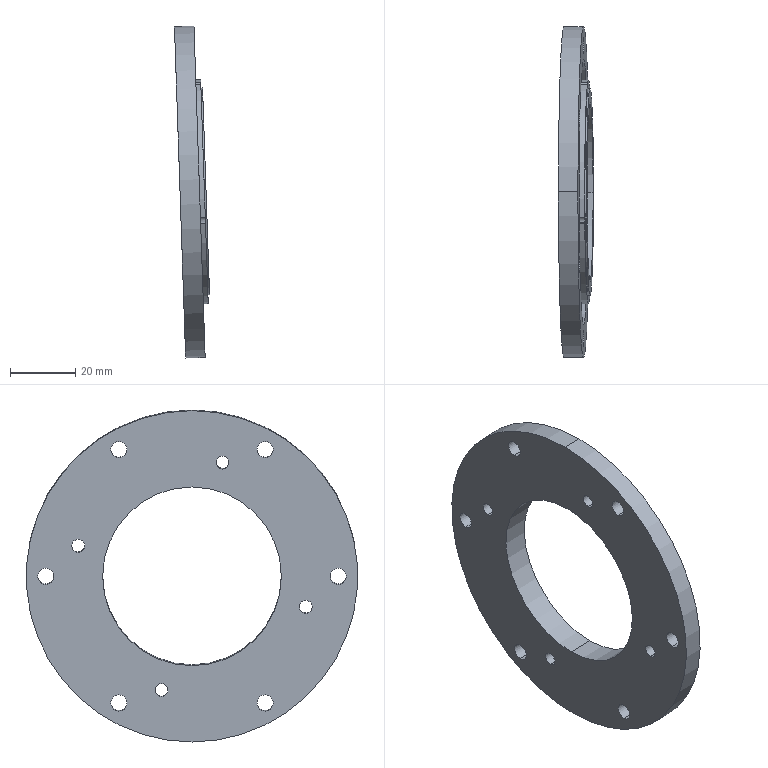Part | STEP file | 2026.6.15-Main Assembly图.sldasm-Part-151 | 1 solid | 38 faces | box 10.798 x 102 x 102.145 mm | volume 33230 mm3 | cylinder 33 | plane 5 | commonest cylinder face diameters 5 x12 4 x8 69 x5 55 x2 63.75 x2 82 x2
STEP:
#1=CARTESIAN_POINT('',(-1696.267,702.018,4104.623));
#2=VERTEX_POINT('',#1);
#3=CARTESIAN_POINT('',(-1695.434,735.086,4079.975));
#4=VERTEX_POINT('',#3);
#5=CARTESIAN_POINT('',(-1696.6,735.086,4114.455));
#6=DIRECTION('',(0.9994,0.,0.03381));
#7=DIRECTION('',(0.01691,0.866,-0.4997));
#8=AXIS2_PLACEMENT_3D('',#5,#6,#7);
#9=CIRCLE('',#8,34.5);
#10=EDGE_CURVE('',#2,#4,#9,.T.);
#11=ORIENTED_EDGE('',*,*,#10,.T.);
#12=CARTESIAN_POINT('',(-1691.936,735.086,4080.093));
#13=VERTEX_POINT('',#12);
#14=CARTESIAN_POINT('',(-1695.434,735.086,4079.975));
#15=DIRECTION('',(0.9994,0.,0.03381));
#16=VECTOR('',#15,1000.);
#17=LINE('',#14,#16);
#18=EDGE_CURVE('',#4,#13,#17,.T.);
#19=ORIENTED_EDGE('',*,*,#18,.T.);
#20=CARTESIAN_POINT('',(-1692.769,702.018,4104.741));
#21=VERTEX_POINT('',#20);
#22=CARTESIAN_POINT('',(-1693.102,735.086,4114.574));
#23=DIRECTION('',(0.9994,0.,0.03381));
#24=DIRECTION('',(-0.03381,0.,0.9994));
#25=AXIS2_PLACEMENT_3D('',#22,#23,#24);
#26=CIRCLE('',#25,34.5);
#27=EDGE_CURVE('',#21,#13,#26,.T.);
#28=ORIENTED_EDGE('',*,*,#27,.F.);
#29=CARTESIAN_POINT('',(-1694.269,702.018,4104.69));
#30=DIRECTION('',(0.9994,0.,0.03381));
#31=VECTOR('',#30,1000.);
#32=LINE('',#29,#31);
#33=EDGE_CURVE('',#2,#21,#32,.T.);
#34=ORIENTED_EDGE('',*,*,#33,.F.);
#35=EDGE_LOOP('',(#11,#19,#28,#34));
#36=FACE_OUTER_BOUND('',#35,.T.);
#37=CARTESIAN_POINT('',(-1696.6,735.086,4114.455));
#38=DIRECTION('',(0.9994,0.,0.03381));
#39=DIRECTION('',(0.03381,0.,-0.9994));
#40=AXIS2_PLACEMENT_3D('',#37,#38,#39);
#41=CYLINDRICAL_SURFACE('',#40,34.5);
#42=ADVANCED_FACE('',(#36),#41,.T.);
#43=CARTESIAN_POINT('',(-1695.214,735.086,4073.479));
#44=VERTEX_POINT('',#43);
#45=CARTESIAN_POINT('',(-1697.986,735.086,4155.432));
#46=VERTEX_POINT('',#45);
#47=CARTESIAN_POINT('',(-1696.6,735.086,4114.455));
#48=DIRECTION('',(-0.9994,0.,-0.03381));
#49=DIRECTION('',(0.01691,0.866,-0.4997));
#50=AXIS2_PLACEMENT_3D('',#47,#48,#49);
#51=CIRCLE('',#50,41.);
#52=EDGE_CURVE('',#44,#46,#51,.T.);
#53=ORIENTED_EDGE('',*,*,#52,.T.);
#54=CARTESIAN_POINT('',(-1695.988,735.086,4155.5));
#55=VERTEX_POINT('',#54);
#56=CARTESIAN_POINT('',(-1697.986,735.086,4155.432));
#57=DIRECTION('',(0.9994,0.,0.03381));
#58=VECTOR('',#57,1000.);
#59=LINE('',#56,#58);
#60=EDGE_CURVE('',#46,#55,#59,.T.);
#61=ORIENTED_EDGE('',*,*,#60,.T.);
#62=CARTESIAN_POINT('',(-1693.215,735.086,4073.546));
#63=VERTEX_POINT('',#62);
#64=CARTESIAN_POINT('',(-1694.601,735.086,4114.523));
#65=DIRECTION('',(0.9994,0.,0.03381));
#66=DIRECTION('',(0.01691,0.866,-0.4997));
#67=AXIS2_PLACEMENT_3D('',#64,#65,#66);
#68=CIRCLE('',#67,41.);
#69=EDGE_CURVE('',#55,#63,#68,.T.);
#70=ORIENTED_EDGE('',*,*,#69,.T.);
#71=CARTESIAN_POINT('',(-1695.214,735.086,4073.479));
#72=DIRECTION('',(0.9994,0.,0.03381));
#73=VECTOR('',#72,1000.);
#74=LINE('',#71,#73);
#75=EDGE_CURVE('',#44,#63,#74,.T.);
#76=ORIENTED_EDGE('',*,*,#75,.F.);
#77=EDGE_LOOP('',(#53,#61,#70,#76));
#78=FACE_OUTER_BOUND('',#77,.T.);
#79=CARTESIAN_POINT('',(-1696.6,735.086,4114.455));
#80=DIRECTION('',(0.9994,0.,0.03381));
#81=DIRECTION('',(0.03381,0.,-0.9994));
#82=AXIS2_PLACEMENT_3D('',#79,#80,#81);
#83=CYLINDRICAL_SURFACE('',#82,41.);
#84=ADVANCED_FACE('',(#78),#83,.F.);
#85=CARTESIAN_POINT('',(-1691.525,735.086,4082.734));
#86=VERTEX_POINT('',#85);
#87=CARTESIAN_POINT('',(-1693.68,735.086,4146.447));
#88=VERTEX_POINT('',#87);
#89=CARTESIAN_POINT('',(-1692.602,735.086,4114.591));
#90=DIRECTION('',(0.9994,0.,0.03381));
#91=DIRECTION('',(0.01691,0.866,-0.4997));
#92=AXIS2_PLACEMENT_3D('',#89,#90,#91);
#93=CIRCLE('',#92,31.875);
#94=EDGE_CURVE('',#86,#88,#93,.T.);
#95=ORIENTED_EDGE('',*,*,#94,.F.);
#96=CARTESIAN_POINT('',(-1692.024,735.086,4082.717));
#97=VERTEX_POINT('',#96);
#98=CARTESIAN_POINT('',(-1691.525,735.086,4082.734));
#99=DIRECTION('',(-0.9994,0.,-0.03381));
#100=VECTOR('',#99,1000.);
#101=LINE('',#98,#100);
#102=EDGE_CURVE('',#86,#97,#101,.T.);
#103=ORIENTED_EDGE('',*,*,#102,.T.);
#104=CARTESIAN_POINT('',(-1694.18,735.086,4146.43));
#105=VERTEX_POINT('',#104);
#106=CARTESIAN_POINT('',(-1693.102,735.086,4114.574));
#107=DIRECTION('',(-0.9994,0.,-0.03381));
#108=DIRECTION('',(0.01691,0.866,-0.4997));
#109=AXIS2_PLACEMENT_3D('',#106,#107,#108);
#110=CIRCLE('',#109,31.875);
#111=EDGE_CURVE('',#105,#97,#110,.T.);
#112=ORIENTED_EDGE('',*,*,#111,.F.);
#113=CARTESIAN_POINT('',(-1693.68,735.086,4146.447));
#114=DIRECTION('',(-0.9994,0.,-0.03381));
#115=VECTOR('',#114,1000.);
#116=LINE('',#113,#115);
#117=EDGE_CURVE('',#88,#105,#116,.T.);
#118=ORIENTED_EDGE('',*,*,#117,.F.);
#119=EDGE_LOOP('',(#95,#103,#112,#118));
#120=FACE_OUTER_BOUND('',#119,.T.);
#121=CARTESIAN_POINT('',(-1692.602,735.086,4114.591));
#122=DIRECTION('',(-0.9994,0.,-0.03381));
#123=DIRECTION('',(-0.03381,0.,0.9994));
#124=AXIS2_PLACEMENT_3D('',#121,#122,#123);
#125=CYLINDRICAL_SURFACE('',#124,31.875);
#126=ADVANCED_FACE('',(#120),#125,.T.);
#127=CARTESIAN_POINT('',(-1696.004,757.586,4155.97));
#128=VERTEX_POINT('',#127);
#129=CARTESIAN_POINT('',(-1695.834,757.586,4150.973));
#130=VERTEX_POINT('',#129);
#131=CARTESIAN_POINT('',(-1695.919,757.586,4153.472));
#132=DIRECTION('',(0.9994,0.,0.03381));
#133=DIRECTION('',(-0.03381,0.,0.9994));
#134=AXIS2_PLACEMENT_3D('',#131,#132,#133);
#135=CIRCLE('',#134,2.5);
#136=EDGE_CURVE('',#128,#130,#135,.T.);
#137=ORIENTED_EDGE('',*,*,#136,.T.);
#138=CARTESIAN_POINT('',(-1701.831,757.586,4150.77));
#139=VERTEX_POINT('',#138);
#140=CARTESIAN_POINT('',(-1693.836,757.586,4151.041));
#141=DIRECTION('',(-0.9994,0.,-0.03381));
#142=VECTOR('',#141,1000.);
#143=LINE('',#140,#142);
#144=EDGE_CURVE('',#130,#139,#143,.T.);
#145=ORIENTED_EDGE('',*,*,#144,.T.);
#146=CARTESIAN_POINT('',(-1702.,757.586,4155.768));
#147=VERTEX_POINT('',#146);
#148=CARTESIAN_POINT('',(-1701.916,757.586,4153.269));
#149=DIRECTION('',(-0.9994,0.,-0.03381));
#150=DIRECTION('',(-0.01691,-0.866,0.4997));
#151=AXIS2_PLACEMENT_3D('',#148,#149,#150);
#152=CIRCLE('',#151,2.5);
#153=EDGE_CURVE('',#139,#147,#152,.T.);
#154=ORIENTED_EDGE('',*,*,#153,.T.);
#155=CARTESIAN_POINT('',(-1694.005,757.586,4156.038));
#156=DIRECTION('',(-0.9994,0.,-0.03381));
#157=VECTOR('',#156,1000.);
#158=LINE('',#155,#157);
#159=EDGE_CURVE('',#128,#147,#158,.T.);
#160=ORIENTED_EDGE('',*,*,#159,.F.);
#161=EDGE_LOOP('',(#137,#145,#154,#160));
#162=FACE_OUTER_BOUND('',#161,.T.);
#163=CARTESIAN_POINT('',(-1693.92,757.586,4153.539));
#164=DIRECTION('',(-0.9994,0.,-0.03381));
#165=DIRECTION('',(-0.03381,0.,0.9994));
#166=AXIS2_PLACEMENT_3D('',#163,#164,#165);
#167=CYLINDRICAL_SURFACE('',#166,2.5);
#168=ADVANCED_FACE('',(#162),#167,.F.);
#169=CARTESIAN_POINT('',(-1696.326,735.086,4165.494));
#170=VERTEX_POINT('',#169);
#171=CARTESIAN_POINT('',(-1692.877,735.086,4063.552));
#172=VERTEX_POINT('',#171);
#173=CARTESIAN_POINT('',(-1694.601,735.086,4114.523));
#174=DIRECTION('',(-0.9994,0.,-0.03381));
#175=DIRECTION('',(-0.03381,0.,0.9994));
#176=AXIS2_PLACEMENT_3D('',#173,#174,#175);
#177=CIRCLE('',#176,51.);
#178=EDGE_CURVE('',#170,#172,#177,.T.);
#179=ORIENTED_EDGE('',*,*,#178,.T.);
#180=CARTESIAN_POINT('',(-1698.873,735.086,4063.349));
#181=VERTEX_POINT('',#180);
#182=CARTESIAN_POINT('',(-1690.878,735.086,4063.62));
#183=DIRECTION('',(-0.9994,0.,-0.03381));
#184=VECTOR('',#183,1000.);
#185=LINE('',#182,#184);
#186=EDGE_CURVE('',#172,#181,#185,.T.);
#187=ORIENTED_EDGE('',*,*,#186,.T.);
#188=CARTESIAN_POINT('',(-1702.322,735.086,4165.291));
#189=VERTEX_POINT('',#188);
#190=CARTESIAN_POINT('',(-1700.598,735.086,4114.32));
#191=DIRECTION('',(0.9994,0.,0.03381));
#192=DIRECTION('',(0.01691,0.866,-0.4997));
#193=AXIS2_PLACEMENT_3D('',#190,#191,#192);
#194=CIRCLE('',#193,51.);
#195=EDGE_CURVE('',#181,#189,#194,.T.);
#196=ORIENTED_EDGE('',*,*,#195,.T.);
#197=CARTESIAN_POINT('',(-1694.327,735.086,4165.561));
#198=DIRECTION('',(-0.9994,0.,-0.03381));
#199=VECTOR('',#198,1000.);
#200=LINE('',#197,#199);
#201=EDGE_CURVE('',#170,#189,#200,.T.);
#202=ORIENTED_EDGE('',*,*,#201,.F.);
#203=EDGE_LOOP('',(#179,#187,#196,#202));
#204=FACE_OUTER_BOUND('',#203,.T.);
#205=CARTESIAN_POINT('',(-1692.602,735.086,4114.591));
#206=DIRECTION('',(-0.9994,0.,-0.03381));
#207=DIRECTION('',(-0.03381,0.,0.9994));
#208=AXIS2_PLACEMENT_3D('',#205,#206,#207);
#209=CYLINDRICAL_SURFACE('',#208,51.);
#210=ADVANCED_FACE('',(#204),#209,.T.);
#211=CARTESIAN_POINT('',(-1696.004,712.586,4155.97));
#212=VERTEX_POINT('',#211);
#213=CARTESIAN_POINT('',(-1695.834,712.586,4150.973));
#214=VERTEX_POINT('',#213);
#215=CARTESIAN_POINT('',(-1695.919,712.586,4153.472));
#216=DIRECTION('',(0.9994,0.,0.03381));
#217=DIRECTION('',(-0.03381,0.,0.9994));
#218=AXIS2_PLACEMENT_3D('',#215,#216,#217);
#219=CIRCLE('',#218,2.5);
#220=EDGE_CURVE('',#212,#214,#219,.T.);
#221=ORIENTED_EDGE('',*,*,#220,.T.);
#222=CARTESIAN_POINT('',(-1701.831,712.586,4150.77));
#223=VERTEX_POINT('',#222);
#224=CARTESIAN_POINT('',(-1693.836,712.586,4151.041));
#225=DIRECTION('',(-0.9994,0.,-0.03381));
#226=VECTOR('',#225,1000.);
#227=LINE('',#224,#226);
#228=EDGE_CURVE('',#214,#223,#227,.T.);
#229=ORIENTED_EDGE('',*,*,#228,.T.);
#230=CARTESIAN_POINT('',(-1702.,712.586,4155.768));
#231=VERTEX_POINT('',#230);
#232=CARTESIAN_POINT('',(-1701.916,712.586,4153.269));
#233=DIRECTION('',(-0.9994,0.,-0.03381));
#234=DIRECTION('',(-0.01691,-0.866,0.4997));
#235=AXIS2_PLACEMENT_3D('',#232,#233,#234);
#236=CIRCLE('',#235,2.5);
#237=EDGE_CURVE('',#223,#231,#236,.T.);
#238=ORIENTED_EDGE('',*,*,#237,.T.);
#239=CARTESIAN_POINT('',(-1694.005,712.586,4156.038));
#240=DIRECTION('',(-0.9994,0.,-0.03381));
#241=VECTOR('',#240,1000.);
#242=LINE('',#239,#241);
#243=EDGE_CURVE('',#212,#231,#242,.T.);
#244=ORIENTED_EDGE('',*,*,#243,.F.);
#245=EDGE_LOOP('',(#221,#229,#238,#244));
#246=FACE_OUTER_BOUND('',#245,.T.);
#247=CARTESIAN_POINT('',(-1693.92,712.586,4153.539));
#248=DIRECTION('',(-0.9994,0.,-0.03381));
#249=DIRECTION('',(-0.03381,0.,0.9994));
#250=AXIS2_PLACEMENT_3D('',#247,#248,#249);
#251=CYLINDRICAL_SURFACE('',#250,2.5);
#252=ADVANCED_FACE('',(#246),#251,.F.);
#253=CARTESIAN_POINT('',(-1696.85,770.101,4121.833));
#254=VERTEX_POINT('',#253);
#255=CARTESIAN_POINT('',(-1696.871,768.642,4122.464));
#256=VERTEX_POINT('',#255);
#257=CARTESIAN_POINT('',(-1696.917,770.101,4123.832));
#258=DIRECTION('',(-0.9994,0.,-0.03381));
#259=DIRECTION('',(0.03381,0.,-0.9994));
#260=AXIS2_PLACEMENT_3D('',#257,#258,#259);
#261=CIRCLE('',#260,2.);
#262=EDGE_CURVE('',#254,#256,#261,.T.);
#263=ORIENTED_EDGE('',*,*,#262,.F.);
#264=CARTESIAN_POINT('',(-1700.847,770.101,4121.698));
#265=VERTEX_POINT('',#264);
#266=CARTESIAN_POINT('',(-1692.852,770.101,4121.969));
#267=DIRECTION('',(-0.9994,0.,-0.03381));
#268=VECTOR('',#267,1000.);
#269=LINE('',#266,#268);
#270=EDGE_CURVE('',#254,#265,#269,.T.);
#271=ORIENTED_EDGE('',*,*,#270,.T.);
#272=CARTESIAN_POINT('',(-1700.983,770.101,4125.696));
#273=VERTEX_POINT('',#272);
#274=CARTESIAN_POINT('',(-1700.915,770.101,4123.697));
#275=DIRECTION('',(-0.9994,0.,-0.03381));
#276=DIRECTION('',(-0.01691,-0.866,0.4997));
#277=AXIS2_PLACEMENT_3D('',#274,#275,#276);
#278=CIRCLE('',#277,2.);
#279=EDGE_CURVE('',#265,#273,#278,.T.);
#280=ORIENTED_EDGE('',*,*,#279,.T.);
#281=CARTESIAN_POINT('',(-1696.985,770.101,4125.831));
#282=VERTEX_POINT('',#281);
#283=CARTESIAN_POINT('',(-1692.987,770.101,4125.966));
#284=DIRECTION('',(-0.9994,0.,-0.03381));
#285=VECTOR('',#284,1000.);
#286=LINE('',#283,#285);
#287=EDGE_CURVE('',#282,#273,#286,.T.);
#288=ORIENTED_EDGE('',*,*,#287,.F.);
#289=CARTESIAN_POINT('',(-1696.933,768.153,4124.288));
#290=VERTEX_POINT('',#289);
#291=CARTESIAN_POINT('',(-1696.917,770.101,4123.832));
#292=DIRECTION('',(-0.9994,0.,-0.03381));
#293=DIRECTION('',(0.03381,0.,-0.9994));
#294=AXIS2_PLACEMENT_3D('',#291,#292,#293);
#295=CIRCLE('',#294,2.);
#296=EDGE_CURVE('',#290,#282,#295,.T.);
#297=ORIENTED_EDGE('',*,*,#296,.F.);
#298=CARTESIAN_POINT('',(-1693.435,768.153,4124.406));
#299=VERTEX_POINT('',#298);
#300=CARTESIAN_POINT('',(-1694.934,768.153,4124.356));
#301=DIRECTION('',(0.9994,0.,0.03381));
#302=VECTOR('',#301,1000.);
#303=LINE('',#300,#302);
#304=EDGE_CURVE('',#290,#299,#303,.T.);
#305=ORIENTED_EDGE('',*,*,#304,.T.);
#306=CARTESIAN_POINT('',(-1693.373,768.642,4122.583));
#307=VERTEX_POINT('',#306);
#308=CARTESIAN_POINT('',(-1693.419,770.101,4123.951));
#309=DIRECTION('',(0.9994,0.,0.03381));
#310=DIRECTION('',(-0.03381,0.,0.9994));
#311=AXIS2_PLACEMENT_3D('',#308,#309,#310);
#312=CIRCLE('',#311,2.);
#313=EDGE_CURVE('',#299,#307,#312,.T.);
#314=ORIENTED_EDGE('',*,*,#313,.T.);
#315=CARTESIAN_POINT('',(-1694.872,768.642,4122.532));
#316=DIRECTION('',(-0.9994,0.,-0.03381));
#317=VECTOR('',#316,1000.);
#318=LINE('',#315,#317);
#319=EDGE_CURVE('',#307,#256,#318,.T.);
#320=ORIENTED_EDGE('',*,*,#319,.T.);
#321=EDGE_LOOP('',(#263,#271,#280,#288,#297,#305,#314,#320));
#322=FACE_OUTER_BOUND('',#321,.T.);
#323=CARTESIAN_POINT('',(-1692.92,770.101,4123.967));
#324=DIRECTION('',(-0.9994,0.,-0.03381));
#325=DIRECTION('',(-0.03381,0.,0.9994));
#326=AXIS2_PLACEMENT_3D('',#323,#324,#325);
#327=CYLINDRICAL_SURFACE('',#326,2.);
#328=ADVANCED_FACE('',(#322),#327,.F.);
#329=CARTESIAN_POINT('',(-1694.686,690.086,4117.022));
#330=VERTEX_POINT('',#329);
#331=CARTESIAN_POINT('',(-1694.517,690.086,4112.024));
#332=VERTEX_POINT('',#331);
#333=CARTESIAN_POINT('',(-1694.601,690.086,4114.523));
#334=DIRECTION('',(0.9994,0.,0.03381));
#335=DIRECTION('',(-0.03381,0.,0.9994));
#336=AXIS2_PLACEMENT_3D('',#333,#334,#335);
#337=CIRCLE('',#336,2.5);
#338=EDGE_CURVE('',#330,#332,#337,.T.);
#339=ORIENTED_EDGE('',*,*,#338,.T.);
#340=CARTESIAN_POINT('',(-1700.513,690.086,4111.822));
#341=VERTEX_POINT('',#340);
#342=CARTESIAN_POINT('',(-1692.518,690.086,4112.092));
#343=DIRECTION('',(-0.9994,0.,-0.03381));
#344=VECTOR('',#343,1000.);
#345=LINE('',#342,#344);
#346=EDGE_CURVE('',#332,#341,#345,.T.);
#347=ORIENTED_EDGE('',*,*,#346,.T.);
#348=CARTESIAN_POINT('',(-1700.682,690.086,4116.819));
#349=VERTEX_POINT('',#348);
#350=CARTESIAN_POINT('',(-1700.598,690.086,4114.32));
#351=DIRECTION('',(-0.9994,0.,-0.03381));
#352=DIRECTION('',(-0.01691,-0.866,0.4997));
#353=AXIS2_PLACEMENT_3D('',#350,#351,#352);
#354=CIRCLE('',#353,2.5);
#355=EDGE_CURVE('',#341,#349,#354,.T.);
#356=ORIENTED_EDGE('',*,*,#355,.T.);
#357=CARTESIAN_POINT('',(-1692.687,690.086,4117.089));
#358=DIRECTION('',(-0.9994,0.,-0.03381));
#359=VECTOR('',#358,1000.);
#360=LINE('',#357,#359);
#361=EDGE_CURVE('',#330,#349,#360,.T.);
#362=ORIENTED_EDGE('',*,*,#361,.F.);
#363=EDGE_LOOP('',(#339,#347,#356,#362));
#364=FACE_OUTER_BOUND('',#363,.T.);
#365=CARTESIAN_POINT('',(-1692.602,690.086,4114.591));
#366=DIRECTION('',(-0.9994,0.,-0.03381));
#367=DIRECTION('',(-0.03381,0.,0.9994));
#368=AXIS2_PLACEMENT_3D('',#365,#366,#367);
#369=CYLINDRICAL_SURFACE('',#368,2.5);
#370=ADVANCED_FACE('',(#364),#369,.F.);
#371=CARTESIAN_POINT('',(-1691.673,735.086,4087.106));
#372=VERTEX_POINT('',#371);
#373=CARTESIAN_POINT('',(-1693.532,735.086,4142.075));
#374=VERTEX_POINT('',#373);
#375=CARTESIAN_POINT('',(-1692.602,735.086,4114.591));
#376=DIRECTION('',(-0.9994,0.,-0.03381));
#377=DIRECTION('',(-0.01691,-0.866,0.4997));
#378=AXIS2_PLACEMENT_3D('',#375,#376,#377);
#379=CIRCLE('',#378,27.5);
#380=EDGE_CURVE('',#372,#374,#379,.T.);
#381=ORIENTED_EDGE('',*,*,#380,.F.);
#382=CARTESIAN_POINT('',(-1699.668,735.086,4086.836));
#383=VERTEX_POINT('',#382);
#384=CARTESIAN_POINT('',(-1691.673,735.086,4087.106));
#385=DIRECTION('',(-0.9994,0.,-0.03381));
#386=VECTOR('',#385,1000.);
#387=LINE('',#384,#386);
#388=EDGE_CURVE('',#372,#383,#387,.T.);
#389=ORIENTED_EDGE('',*,*,#388,.T.);
#390=CARTESIAN_POINT('',(-1701.528,735.086,4141.804));
#391=VERTEX_POINT('',#390);
#392=CARTESIAN_POINT('',(-1700.598,735.086,4114.32));
#393=DIRECTION('',(-0.9994,0.,-0.03381));
#394=DIRECTION('',(-0.01691,-0.866,0.4997));
#395=AXIS2_PLACEMENT_3D('',#392,#393,#394);
#396=CIRCLE('',#395,27.5);
#397=EDGE_CURVE('',#383,#391,#396,.T.);
#398=ORIENTED_EDGE('',*,*,#397,.T.);
#399=CARTESIAN_POINT('',(-1693.532,735.086,4142.075));
#400=DIRECTION('',(-0.9994,0.,-0.03381));
#401=VECTOR('',#400,1000.);
#402=LINE('',#399,#401);
#403=EDGE_CURVE('',#374,#391,#402,.T.);
#404=ORIENTED_EDGE('',*,*,#403,.F.);
#405=EDGE_LOOP('',(#381,#389,#398,#404));
#406=FACE_OUTER_BOUND('',#405,.T.);
#407=CARTESIAN_POINT('',(-1692.602,735.086,4114.591));
#408=DIRECTION('',(-0.9994,0.,-0.03381));
#409=DIRECTION('',(-0.03381,0.,0.9994));
#410=AXIS2_PLACEMENT_3D('',#407,#408,#409);
#411=CYLINDRICAL_SURFACE('',#410,27.5);
#412=ADVANCED_FACE('',(#406),#411,.F.);
#413=CARTESIAN_POINT('',(-1693.368,757.586,4078.073));
#414=VERTEX_POINT('',#413);
#415=CARTESIAN_POINT('',(-1693.199,757.586,4073.076));
#416=VERTEX_POINT('',#415);
#417=CARTESIAN_POINT('',(-1693.283,757.586,4075.574));
#418=DIRECTION('',(0.9994,0.,0.03381));
#419=DIRECTION('',(-0.03381,0.,0.9994));
#420=AXIS2_PLACEMENT_3D('',#417,#418,#419);
#421=CIRCLE('',#420,2.5);
#422=EDGE_CURVE('',#414,#416,#421,.T.);
#423=ORIENTED_EDGE('',*,*,#422,.T.);
#424=CARTESIAN_POINT('',(-1699.196,757.586,4072.873));
#425=VERTEX_POINT('',#424);
#426=CARTESIAN_POINT('',(-1691.2,757.586,4073.143));
#427=DIRECTION('',(-0.9994,0.,-0.03381));
#428=VECTOR('',#427,1000.);
#429=LINE('',#426,#428);
#430=EDGE_CURVE('',#416,#425,#429,.T.);
#431=ORIENTED_EDGE('',*,*,#430,.T.);
#432=CARTESIAN_POINT('',(-1699.365,757.586,4077.87));
#433=VERTEX_POINT('',#432);
#434=CARTESIAN_POINT('',(-1699.28,757.586,4075.371));
#435=DIRECTION('',(-0.9994,0.,-0.03381));
#436=DIRECTION('',(-0.01691,-0.866,0.4997));
#437=AXIS2_PLACEMENT_3D('',#434,#435,#436);
#438=CIRCLE('',#437,2.5);
#439=EDGE_CURVE('',#425,#433,#438,.T.);
#440=ORIENTED_EDGE('',*,*,#439,.T.);
#441=CARTESIAN_POINT('',(-1691.369,757.586,4078.14));
#442=DIRECTION('',(-0.9994,0.,-0.03381));
#443=VECTOR('',#442,1000.);
#444=LINE('',#441,#443);
#445=EDGE_CURVE('',#414,#433,#444,.T.);
#446=ORIENTED_EDGE('',*,*,#445,.F.);
#447=EDGE_LOOP('',(#423,#431,#440,#446));
#448=FACE_OUTER_BOUND('',#447,.T.);
#449=CARTESIAN_POINT('',(-1691.285,757.586,4075.642));
#450=DIRECTION('',(-0.9994,0.,-0.03381));
#451=DIRECTION('',(-0.03381,0.,0.9994));
#452=AXIS2_PLACEMENT_3D('',#449,#450,#451);
#453=CYLINDRICAL_SURFACE('',#452,2.5);
#454=ADVANCED_FACE('',(#448),#453,.F.);
#455=CARTESIAN_POINT('',(-1693.368,712.586,4078.073));
#456=VERTEX_POINT('',#455);
#457=CARTESIAN_POINT('',(-1693.199,712.586,4073.076));
#458=VERTEX_POINT('',#457);
#459=CARTESIAN_POINT('',(-1693.283,712.586,4075.574));
#460=DIRECTION('',(0.9994,0.,0.03381));
#461=DIRECTION('',(-0.03381,0.,0.9994));
#462=AXIS2_PLACEMENT_3D('',#459,#460,#461);
#463=CIRCLE('',#462,2.5);
#464=EDGE_CURVE('',#456,#458,#463,.T.);
#465=ORIENTED_EDGE('',*,*,#464,.T.);
#466=CARTESIAN_POINT('',(-1699.196,712.586,4072.873));
#467=VERTEX_POINT('',#466);
#468=CARTESIAN_POINT('',(-1691.2,712.586,4073.143));
#469=DIRECTION('',(-0.9994,0.,-0.03381));
#470=VECTOR('',#469,1000.);
#471=LINE('',#468,#470);
#472=EDGE_CURVE('',#458,#467,#471,.T.);
#473=ORIENTED_EDGE('',*,*,#472,.T.);
#474=CARTESIAN_POINT('',(-1699.365,712.586,4077.87));
#475=VERTEX_POINT('',#474);
#476=CARTESIAN_POINT('',(-1699.28,712.586,4075.371));
#477=DIRECTION('',(-0.9994,0.,-0.03381));
#478=DIRECTION('',(-0.01691,-0.866,0.4997));
#479=AXIS2_PLACEMENT_3D('',#476,#477,#478);
#480=CIRCLE('',#479,2.5);
#481=EDGE_CURVE('',#467,#475,#480,.T.);
#482=ORIENTED_EDGE('',*,*,#481,.T.);
#483=CARTESIAN_POINT('',(-1691.369,712.586,4078.14));
#484=DIRECTION('',(-0.9994,0.,-0.03381));
#485=VECTOR('',#484,1000.);
#486=LINE('',#483,#485);
#487=EDGE_CURVE('',#456,#475,#486,.T.);
#488=ORIENTED_EDGE('',*,*,#487,.F.);
#489=EDGE_LOOP('',(#465,#473,#482,#488));
#490=FACE_OUTER_BOUND('',#489,.T.);
#491=CARTESIAN_POINT('',(-1691.285,712.586,4075.642));
#492=DIRECTION('',(-0.9994,0.,-0.03381));
#493=DIRECTION('',(-0.03381,0.,0.9994));
#494=AXIS2_PLACEMENT_3D('',#491,#492,#493);
#495=CYLINDRICAL_SURFACE('',#494,2.5);
#496=ADVANCED_FACE('',(#490),#495,.F.);
#497=CARTESIAN_POINT('',(-1695.348,744.468,4077.462));
#498=VERTEX_POINT('',#497);
#499=CARTESIAN_POINT('',(-1695.465,743.099,4080.918));
#500=VERTEX_POINT('',#499);
#501=CARTESIAN_POINT('',(-1695.416,744.468,4079.461));
#502=DIRECTION('',(-0.9994,0.,-0.03381));
#503=DIRECTION('',(0.03381,0.,-0.9994));
#504=AXIS2_PLACEMENT_3D('',#501,#502,#503);
#505=CIRCLE('',#504,2.);
#506=EDGE_CURVE('',#498,#500,#505,.T.);
#507=ORIENTED_EDGE('',*,*,#506,.F.);
#508=CARTESIAN_POINT('',(-1699.346,744.468,4077.326));
#509=VERTEX_POINT('',#508);
#510=CARTESIAN_POINT('',(-1691.351,744.468,4077.597));
#511=DIRECTION('',(-0.9994,0.,-0.03381));
#512=VECTOR('',#511,1000.);
#513=LINE('',#510,#512);
#514=EDGE_CURVE('',#498,#509,#513,.T.);
#515=ORIENTED_EDGE('',*,*,#514,.T.);
#516=CARTESIAN_POINT('',(-1699.481,744.468,4081.324));
#517=VERTEX_POINT('',#516);
#518=CARTESIAN_POINT('',(-1699.414,744.468,4079.325));
#519=DIRECTION('',(-0.9994,0.,-0.03381));
#520=DIRECTION('',(-0.01691,-0.866,0.4997));
#521=AXIS2_PLACEMENT_3D('',#518,#519,#520);
#522=CIRCLE('',#521,2.);
#523=EDGE_CURVE('',#509,#517,#522,.T.);
#524=ORIENTED_EDGE('',*,*,#523,.T.);
#525=CARTESIAN_POINT('',(-1691.986,744.468,4081.578));
#526=VERTEX_POINT('',#525);
#527=CARTESIAN_POINT('',(-1691.486,744.468,4081.595));
#528=DIRECTION('',(-0.9994,0.,-0.03381));
#529=VECTOR('',#528,1000.);
#530=LINE('',#527,#529);
#531=EDGE_CURVE('',#526,#517,#530,.T.);
#532=ORIENTED_EDGE('',*,*,#531,.F.);
#533=CARTESIAN_POINT('',(-1691.967,743.099,4081.037));
#534=VERTEX_POINT('',#533);
#535=CARTESIAN_POINT('',(-1691.918,744.468,4079.579));
#536=DIRECTION('',(0.9994,0.,0.03381));
#537=DIRECTION('',(-0.03381,0.,0.9994));
#538=AXIS2_PLACEMENT_3D('',#535,#536,#537);
#539=CIRCLE('',#538,2.);
#540=EDGE_CURVE('',#526,#534,#539,.T.);
#541=ORIENTED_EDGE('',*,*,#540,.T.);
#542=CARTESIAN_POINT('',(-1693.467,743.099,4080.986));
#543=DIRECTION('',(-0.9994,0.,-0.03381));
#544=VECTOR('',#543,1000.);
#545=LINE('',#542,#544);
#546=EDGE_CURVE('',#534,#500,#545,.T.);
#547=ORIENTED_EDGE('',*,*,#546,.T.);
#548=EDGE_LOOP('',(#507,#515,#524,#532,#541,#547));
#549=FACE_OUTER_BOUND('',#548,.T.);
#550=CARTESIAN_POINT('',(-1691.418,744.468,4079.596));
#551=DIRECTION('',(-0.9994,0.,-0.03381));
#552=DIRECTION('',(-0.03381,0.,0.9994));
#553=AXIS2_PLACEMENT_3D('',#550,#551,#552);
#554=CYLINDRICAL_SURFACE('',#553,2.);
#555=ADVANCED_FACE('',(#549),#554,.F.);
#556=CARTESIAN_POINT('',(-1696.215,700.071,4103.08));
#557=VERTEX_POINT('',#556);
#558=CARTESIAN_POINT('',(-1696.35,700.071,4107.077));
#559=VERTEX_POINT('',#558);
#560=CARTESIAN_POINT('',(-1696.283,700.071,4105.079));
#561=DIRECTION('',(-0.9994,0.,-0.03381));
#562=DIRECTION('',(0.03381,0.,-0.9994));
#563=AXIS2_PLACEMENT_3D('',#560,#561,#562);
#564=CIRCLE('',#563,2.);
#565=EDGE_CURVE('',#557,#559,#564,.T.);
#566=ORIENTED_EDGE('',*,*,#565,.F.);
#567=CARTESIAN_POINT('',(-1700.213,700.071,4102.944));
#568=VERTEX_POINT('',#567);
#569=CARTESIAN_POINT('',(-1692.218,700.071,4103.215));
#570=DIRECTION('',(-0.9994,0.,-0.03381));
#571=VECTOR('',#570,1000.);
#572=LINE('',#569,#571);
#573=EDGE_CURVE('',#557,#568,#572,.T.);
#574=ORIENTED_EDGE('',*,*,#573,.T.);
#575=CARTESIAN_POINT('',(-1700.348,700.071,4106.942));
#576=VERTEX_POINT('',#575);
#577=CARTESIAN_POINT('',(-1700.281,700.071,4104.943));
#578=DIRECTION('',(-0.9994,0.,-0.03381));
#579=DIRECTION('',(-0.01691,-0.866,0.4997));
#580=AXIS2_PLACEMENT_3D('',#577,#578,#579);
#581=CIRCLE('',#580,2.);
#582=EDGE_CURVE('',#568,#576,#581,.T.);
#583=ORIENTED_EDGE('',*,*,#582,.T.);
#584=CARTESIAN_POINT('',(-1692.353,700.071,4107.213));
#585=DIRECTION('',(-0.9994,0.,-0.03381));
#586=VECTOR('',#585,1000.);
#587=LINE('',#584,#586);
#588=EDGE_CURVE('',#559,#576,#587,.T.);
#589=ORIENTED_EDGE('',*,*,#588,.F.);
#590=EDGE_LOOP('',(#566,#574,#583,#589));
#591=FACE_OUTER_BOUND('',#590,.T.);
#592=CARTESIAN_POINT('',(-1692.285,700.071,4105.214));
#593=DIRECTION('',(-0.9994,0.,-0.03381));
#594=DIRECTION('',(-0.03381,0.,0.9994));
#595=AXIS2_PLACEMENT_3D('',#592,#593,#594);
#596=CYLINDRICAL_SURFACE('',#595,2.);
#597=ADVANCED_FACE('',(#591),#596,.F.);
#598=CARTESIAN_POINT('',(-1694.686,780.086,4117.022));
#599=VERTEX_POINT('',#598);
#600=CARTESIAN_POINT('',(-1694.517,780.086,4112.024));
#601=VERTEX_POINT('',#600);
#602=CARTESIAN_POINT('',(-1694.601,780.086,4114.523));
#603=DIRECTION('',(0.9994,0.,0.03381));
#604=DIRECTION('',(-0.03381,0.,0.9994));
#605=AXIS2_PLACEMENT_3D('',#602,#603,#604);
#606=CIRCLE('',#605,2.5);
#607=EDGE_CURVE('',#599,#601,#606,.T.);
#608=ORIENTED_EDGE('',*,*,#607,.T.);
#609=CARTESIAN_POINT('',(-1700.513,780.086,4111.822));
#610=VERTEX_POINT('',#609);
#611=CARTESIAN_POINT('',(-1692.518,780.086,4112.092));
#612=DIRECTION('',(-0.9994,0.,-0.03381));
#613=VECTOR('',#612,1000.);
#614=LINE('',#611,#613);
#615=EDGE_CURVE('',#601,#610,#614,.T.);
#616=ORIENTED_EDGE('',*,*,#615,.T.);
#617=CARTESIAN_POINT('',(-1700.682,780.086,4116.819));
#618=VERTEX_POINT('',#617);
#619=CARTESIAN_POINT('',(-1700.598,780.086,4114.32));
#620=DIRECTION('',(-0.9994,0.,-0.03381));
#621=DIRECTION('',(-0.01691,-0.866,0.4997));
#622=AXIS2_PLACEMENT_3D('',#619,#620,#621);
#623=CIRCLE('',#622,2.5);
#624=EDGE_CURVE('',#610,#618,#623,.T.);
#625=ORIENTED_EDGE('',*,*,#624,.T.);
#626=CARTESIAN_POINT('',(-1692.687,780.086,4117.089));
#627=DIRECTION('',(-0.9994,0.,-0.03381));
#628=VECTOR('',#627,1000.);
#629=LINE('',#626,#628);
#630=EDGE_CURVE('',#599,#618,#629,.T.);
#631=ORIENTED_EDGE('',*,*,#630,.F.);
#632=EDGE_LOOP('',(#608,#616,#625,#631));
#633=FACE_OUTER_BOUND('',#632,.T.);
#634=CARTESIAN_POINT('',(-1692.602,780.086,4114.591));
#635=DIRECTION('',(-0.9994,0.,-0.03381));
#636=DIRECTION('',(-0.03381,0.,0.9994));
#637=AXIS2_PLACEMENT_3D('',#634,#635,#636);
#638=CYLINDRICAL_SURFACE('',#637,2.5);
#639=ADVANCED_FACE('',(#633),#638,.F.);
#640=CARTESIAN_POINT('',(-1694.22,725.248,4147.622));
#641=VERTEX_POINT('',#640);
#642=CARTESIAN_POINT('',(-1694.218,725.704,4147.57));
#643=VERTEX_POINT('',#642);
#644=CARTESIAN_POINT('',(-1694.286,725.704,4149.569));
#645=DIRECTION('',(0.9994,0.,0.03381));
#646=DIRECTION('',(-0.03381,0.,0.9994));
#647=AXIS2_PLACEMENT_3D('',#644,#645,#646);
#648=CIRCLE('',#647,2.);
#649=EDGE_CURVE('',#641,#643,#648,.T.);
#650=ORIENTED_EDGE('',*,*,#649,.T.);
#651=CARTESIAN_POINT('',(-1701.714,725.704,4147.316));
#652=VERTEX_POINT('',#651);
#653=CARTESIAN_POINT('',(-1693.719,725.704,4147.587));
#654=DIRECTION('',(-0.9994,0.,-0.03381));
#655=VECTOR('',#654,1000.);
#656=LINE('',#653,#655);
#657=EDGE_CURVE('',#643,#652,#656,.T.);
#658=ORIENTED_EDGE('',*,*,#657,.T.);
#659=CARTESIAN_POINT('',(-1701.849,725.704,4151.314));
#660=VERTEX_POINT('',#659);
#661=CARTESIAN_POINT('',(-1701.782,725.704,4149.315));
#662=DIRECTION('',(-0.9994,0.,-0.03381));
#663=DIRECTION('',(-0.01691,-0.866,0.4997));
#664=AXIS2_PLACEMENT_3D('',#661,#662,#663);
#665=CIRCLE('',#664,2.);
#666=EDGE_CURVE('',#652,#660,#665,.T.);
#667=ORIENTED_EDGE('',*,*,#666,.T.);
#668=CARTESIAN_POINT('',(-1697.852,725.704,4151.449));
#669=VERTEX_POINT('',#668);
#670=CARTESIAN_POINT('',(-1693.854,725.704,4151.584));
#671=DIRECTION('',(-0.9994,0.,-0.03381));
#672=VECTOR('',#671,1000.);
#673=LINE('',#670,#672);
#674=EDGE_CURVE('',#669,#660,#673,.T.);
#675=ORIENTED_EDGE('',*,*,#674,.F.);
#676=CARTESIAN_POINT('',(-1697.718,725.248,4147.504));
#677=VERTEX_POINT('',#676);
#678=CARTESIAN_POINT('',(-1697.784,725.704,4149.45));
#679=DIRECTION('',(-0.9994,0.,-0.03381));
#680=DIRECTION('',(0.03381,0.,-0.9994));
#681=AXIS2_PLACEMENT_3D('',#678,#679,#680);
#682=CIRCLE('',#681,2.);
#683=EDGE_CURVE('',#677,#669,#682,.T.);
#684=ORIENTED_EDGE('',*,*,#683,.F.);
#685=CARTESIAN_POINT('',(-1695.719,725.248,4147.572));
#686=DIRECTION('',(0.9994,0.,0.03381));
#687=VECTOR('',#686,1000.);
#688=LINE('',#685,#687);
#689=EDGE_CURVE('',#677,#641,#688,.T.);
#690=ORIENTED_EDGE('',*,*,#689,.T.);
#691=EDGE_LOOP('',(#650,#658,#667,#675,#684,#690));
#692=FACE_OUTER_BOUND('',#691,.T.);
#693=CARTESIAN_POINT('',(-1693.786,725.704,4149.585));
#694=DIRECTION('',(-0.9994,0.,-0.03381));
#695=DIRECTION('',(-0.03381,0.,0.9994));
#696=AXIS2_PLACEMENT_3D('',#693,#694,#695);
#697=CYLINDRICAL_SURFACE('',#696,2.);
#698=ADVANCED_FACE('',(#692),#697,.F.);
#699=ORIENTED_EDGE('',*,*,#111,.T.);
#700=CARTESIAN_POINT('',(-1693.102,735.086,4114.574));
#701=DIRECTION('',(-0.9994,0.,-0.03381));
#702=DIRECTION('',(0.01691,0.866,-0.4997));
#703=AXIS2_PLACEMENT_3D('',#700,#701,#702);
#704=CIRCLE('',#703,31.875);
#705=EDGE_CURVE('',#97,#105,#704,.T.);
#706=ORIENTED_EDGE('',*,*,#705,.T.);
#707=EDGE_LOOP('',(#699,#706));
#708=FACE_BOUND('',#707,.T.);
#709=ORIENTED_EDGE('',*,*,#649,.F.);
#710=CARTESIAN_POINT('',(-1692.831,701.529,4106.565));
#711=VERTEX_POINT('',#710);
#712=CARTESIAN_POINT('',(-1693.102,735.086,4114.574));
#713=DIRECTION('',(0.9994,0.,0.03381));
#714=DIRECTION('',(-0.03381,0.,0.9994));
#715=AXIS2_PLACEMENT_3D('',#712,#713,#714);
#716=CIRCLE('',#715,34.5);
#717=EDGE_CURVE('',#641,#711,#716,.T.);
#718=ORIENTED_EDGE('',*,*,#717,.T.);
#719=CARTESIAN_POINT('',(-1692.785,700.071,4105.197));
#720=DIRECTION('',(0.9994,0.,0.03381));
#721=DIRECTION('',(-0.03381,0.,0.9994));
#722=AXIS2_PLACEMENT_3D('',#719,#720,#721);
#723=CIRCLE('',#722,2.);
#724=EDGE_CURVE('',#21,#711,#723,.T.);
#725=ORIENTED_EDGE('',*,*,#724,.F.);
#726=ORIENTED_EDGE('',*,*,#27,.T.);
#727=CARTESIAN_POINT('',(-1693.102,735.086,4114.574));
#728=DIRECTION('',(0.9994,0.,0.03381));
#729=DIRECTION('',(-0.03381,0.,0.9994));
#730=AXIS2_PLACEMENT_3D('',#727,#728,#729);
#731=CIRCLE('',#730,34.5);
#732=EDGE_CURVE('',#13,#534,#731,.T.);
#733=ORIENTED_EDGE('',*,*,#732,.T.);
#734=ORIENTED_EDGE('',*,*,#540,.F.);
#735=CARTESIAN_POINT('',(-1691.984,744.924,4081.525));
#736=VERTEX_POINT('',#735);
#737=CARTESIAN_POINT('',(-1691.918,744.468,4079.579));
#738=DIRECTION('',(0.9994,0.,0.03381));
#739=DIRECTION('',(-0.03381,0.,0.9994));
#740=AXIS2_PLACEMENT_3D('',#737,#738,#739);
#741=CIRCLE('',#740,2.);
#742=EDGE_CURVE('',#736,#526,#741,.T.);
#743=ORIENTED_EDGE('',*,*,#742,.F.);
#744=CARTESIAN_POINT('',(-1693.102,735.086,4114.574));
#745=DIRECTION('',(0.9994,0.,0.03381));
#746=DIRECTION('',(-0.03381,0.,0.9994));
#747=AXIS2_PLACEMENT_3D('',#744,#745,#746);
#748=CIRCLE('',#747,34.5);
#749=EDGE_CURVE('',#736,#307,#748,.T.);
#750=ORIENTED_EDGE('',*,*,#749,.T.);
#751=ORIENTED_EDGE('',*,*,#313,.F.);
#752=CARTESIAN_POINT('',(-1694.237,727.072,4148.111));
#753=VERTEX_POINT('',#752);
#754=CARTESIAN_POINT('',(-1693.102,735.086,4114.574));
#755=DIRECTION('',(0.9994,0.,0.03381));
#756=DIRECTION('',(-0.03381,0.,0.9994));
#757=AXIS2_PLACEMENT_3D('',#754,#755,#756);
#758=CIRCLE('',#757,34.5);
#759=EDGE_CURVE('',#299,#753,#758,.T.);
#760=ORIENTED_EDGE('',*,*,#759,.T.);
#761=CARTESIAN_POINT('',(-1694.286,725.704,4149.569));
#762=DIRECTION('',(0.9994,0.,0.03381));
#763=DIRECTION('',(-0.03381,0.,0.9994));
#764=AXIS2_PLACEMENT_3D('',#761,#762,#763);
#765=CIRCLE('',#764,2.);
#766=EDGE_CURVE('',#643,#753,#765,.T.);
#767=ORIENTED_EDGE('',*,*,#766,.F.);
#768=EDGE_LOOP('',(#709,#718,#725,#726,#733,#734,#743,#750,#751,#760,#767));
#769=FACE_OUTER_BOUND('',#768,.T.);
#770=CARTESIAN_POINT('',(-1693.102,735.086,4114.574));
#771=DIRECTION('',(-0.9994,0.,-0.03381));
#772=DIRECTION('',(-0.03381,0.,0.9994));
#773=AXIS2_PLACEMENT_3D('',#770,#771,#772);
#774=PLANE('',#773);
#775=ADVANCED_FACE('',(#708,#769),#774,.F.);
#776=CARTESIAN_POINT('',(-1692.602,735.086,4114.591));
#777=DIRECTION('',(-0.9994,0.,-0.03381));
#778=DIRECTION('',(-0.01691,-0.866,0.4997));
#779=AXIS2_PLACEMENT_3D('',#776,#777,#778);
#780=CIRCLE('',#779,27.5);
#781=EDGE_CURVE('',#374,#372,#780,.T.);
#782=ORIENTED_EDGE('',*,*,#781,.T.);
#783=ORIENTED_EDGE('',*,*,#380,.T.);
#784=EDGE_LOOP('',(#782,#783));
#785=FACE_BOUND('',#784,.T.);
#786=CARTESIAN_POINT('',(-1692.602,735.086,4114.591));
#787=DIRECTION('',(0.9994,0.,0.03381));
#788=DIRECTION('',(0.01691,0.866,-0.4997));
#789=AXIS2_PLACEMENT_3D('',#786,#787,#788);
#790=CIRCLE('',#789,31.875);
#791=EDGE_CURVE('',#88,#86,#790,.T.);
#792=ORIENTED_EDGE('',*,*,#791,.T.);
#793=ORIENTED_EDGE('',*,*,#94,.T.);
#794=EDGE_LOOP('',(#792,#793));
#795=FACE_OUTER_BOUND('',#794,.T.);
#796=CARTESIAN_POINT('',(-1693.261,723.836,4134.065));
#797=DIRECTION('',(0.9994,0.,0.03381));
#798=DIRECTION('',(0.03381,0.,-0.9994));
#799=AXIS2_PLACEMENT_3D('',#796,#797,#798);
#800=PLANE('',#799);
#801=ADVANCED_FACE('',(#785,#795),#800,.T.);
#802=ORIENTED_EDGE('',*,*,#657,.F.);
#803=ORIENTED_EDGE('',*,*,#766,.T.);
#804=CARTESIAN_POINT('',(-1697.735,727.072,4147.993));
#805=VERTEX_POINT('',#804);
#806=CARTESIAN_POINT('',(-1695.736,727.072,4148.06));
#807=DIRECTION('',(-0.9994,0.,-0.03381));
#808=VECTOR('',#807,1000.);
#809=LINE('',#806,#808);
#810=EDGE_CURVE('',#753,#805,#809,.T.);
#811=ORIENTED_EDGE('',*,*,#810,.T.);
#812=CARTESIAN_POINT('',(-1697.784,725.704,4149.45));
#813=DIRECTION('',(-0.9994,0.,-0.03381));
#814=DIRECTION('',(0.03381,0.,-0.9994));
#815=AXIS2_PLACEMENT_3D('',#812,#813,#814);
#816=CIRCLE('',#815,2.);
#817=EDGE_CURVE('',#669,#805,#816,.T.);
#818=ORIENTED_EDGE('',*,*,#817,.F.);
#819=ORIENTED_EDGE('',*,*,#674,.T.);
#820=CARTESIAN_POINT('',(-1701.782,725.704,4149.315));
#821=DIRECTION('',(-0.9994,0.,-0.03381));
#822=DIRECTION('',(-0.01691,-0.866,0.4997));
#823=AXIS2_PLACEMENT_3D('',#820,#821,#822);
#824=CIRCLE('',#823,2.);
#825=EDGE_CURVE('',#660,#652,#824,.T.);
#826=ORIENTED_EDGE('',*,*,#825,.T.);
#827=EDGE_LOOP('',(#802,#803,#811,#818,#819,#826));
#828=FACE_OUTER_BOUND('',#827,.T.);
#829=CARTESIAN_POINT('',(-1693.786,725.704,4149.585));
#830=DIRECTION('',(-0.9994,0.,-0.03381));
#831=DIRECTION('',(-0.03381,0.,0.9994));
#832=AXIS2_PLACEMENT_3D('',#829,#830,#831);
#833=CYLINDRICAL_SURFACE('',#832,2.);
#834=ADVANCED_FACE('',(#828),#833,.F.);
#835=ORIENTED_EDGE('',*,*,#615,.F.);
#836=CARTESIAN_POINT('',(-1694.601,780.086,4114.523));
#837=DIRECTION('',(0.9994,0.,0.03381));
#838=DIRECTION('',(-0.03381,0.,0.9994));
#839=AXIS2_PLACEMENT_3D('',#836,#837,#838);
#840=CIRCLE('',#839,2.5);
#841=EDGE_CURVE('',#601,#599,#840,.T.);
#842=ORIENTED_EDGE('',*,*,#841,.T.);
#843=ORIENTED_EDGE('',*,*,#630,.T.);
#844=CARTESIAN_POINT('',(-1700.598,780.086,4114.32));
#845=DIRECTION('',(-0.9994,0.,-0.03381));
#846=DIRECTION('',(-0.01691,-0.866,0.4997));
#847=AXIS2_PLACEMENT_3D('',#844,#845,#846);
#848=CIRCLE('',#847,2.5);
#849=EDGE_CURVE('',#618,#610,#848,.T.);
#850=ORIENTED_EDGE('',*,*,#849,.T.);
#851=EDGE_LOOP('',(#835,#842,#843,#850));
#852=FACE_OUTER_BOUND('',#851,.T.);
#853=CARTESIAN_POINT('',(-1692.602,780.086,4114.591));
#854=DIRECTION('',(-0.9994,0.,-0.03381));
#855=DIRECTION('',(-0.03381,0.,0.9994));
#856=AXIS2_PLACEMENT_3D('',#853,#854,#855);
#857=CYLINDRICAL_SURFACE('',#856,2.5);
#858=ADVANCED_FACE('',(#852),#857,.F.);
#859=ORIENTED_EDGE('',*,*,#573,.F.);
#860=CARTESIAN_POINT('',(-1696.283,700.071,4105.079));
#861=DIRECTION('',(-0.9994,0.,-0.03381));
#862=DIRECTION('',(0.03381,0.,-0.9994));
#863=AXIS2_PLACEMENT_3D('',#860,#861,#862);
#864=CIRCLE('',#863,2.);
#865=EDGE_CURVE('',#2,#557,#864,.T.);
#866=ORIENTED_EDGE('',*,*,#865,.F.);
#867=ORIENTED_EDGE('',*,*,#33,.T.);
#868=ORIENTED_EDGE('',*,*,#724,.T.);
#869=CARTESIAN_POINT('',(-1696.329,701.529,4106.446));
#870=VERTEX_POINT('',#869);
#871=CARTESIAN_POINT('',(-1694.33,701.529,4106.514));
#872=DIRECTION('',(-0.9994,0.,-0.03381));
#873=VECTOR('',#872,1000.);
#874=LINE('',#871,#873);
#875=EDGE_CURVE('',#711,#870,#874,.T.);
#876=ORIENTED_EDGE('',*,*,#875,.T.);
#877=CARTESIAN_POINT('',(-1696.283,700.071,4105.079));
#878=DIRECTION('',(-0.9994,0.,-0.03381));
#879=DIRECTION('',(0.03381,0.,-0.9994));
#880=AXIS2_PLACEMENT_3D('',#877,#878,#879);
#881=CIRCLE('',#880,2.);
#882=EDGE_CURVE('',#559,#870,#881,.T.);
#883=ORIENTED_EDGE('',*,*,#882,.F.);
#884=ORIENTED_EDGE('',*,*,#588,.T.);
#885=CARTESIAN_POINT('',(-1700.281,700.071,4104.943));
#886=DIRECTION('',(-0.9994,0.,-0.03381));
#887=DIRECTION('',(-0.01691,-0.866,0.4997));
#888=AXIS2_PLACEMENT_3D('',#885,#886,#887);
#889=CIRCLE('',#888,2.);
#890=EDGE_CURVE('',#576,#568,#889,.T.);
#891=ORIENTED_EDGE('',*,*,#890,.T.);
#892=EDGE_LOOP('',(#859,#866,#867,#868,#876,#883,#884,#891));
#893=FACE_OUTER_BOUND('',#892,.T.);
#894=CARTESIAN_POINT('',(-1692.285,700.071,4105.214));
#895=DIRECTION('',(-0.9994,0.,-0.03381));
#896=DIRECTION('',(-0.03381,0.,0.9994));
#897=AXIS2_PLACEMENT_3D('',#894,#895,#896);
#898=CYLINDRICAL_SURFACE('',#897,2.);
#899=ADVANCED_FACE('',(#893),#898,.F.);
#900=ORIENTED_EDGE('',*,*,#514,.F.);
#901=CARTESIAN_POINT('',(-1695.482,744.924,4081.407));
#902=VERTEX_POINT('',#901);
#903=CARTESIAN_POINT('',(-1695.416,744.468,4079.461));
#904=DIRECTION('',(-0.9994,0.,-0.03381));
#905=DIRECTION('',(0.03381,0.,-0.9994));
#906=AXIS2_PLACEMENT_3D('',#903,#904,#905);
#907=CIRCLE('',#906,2.);
#908=EDGE_CURVE('',#902,#498,#907,.T.);
#909=ORIENTED_EDGE('',*,*,#908,.F.);
#910=CARTESIAN_POINT('',(-1693.483,744.924,4081.474));
#911=DIRECTION('',(0.9994,0.,0.03381));
#912=VECTOR('',#911,1000.);
#913=LINE('',#910,#912);
#914=EDGE_CURVE('',#902,#736,#913,.T.);
#915=ORIENTED_EDGE('',*,*,#914,.T.);
#916=ORIENTED_EDGE('',*,*,#742,.T.);
#917=ORIENTED_EDGE('',*,*,#531,.T.);
#918=CARTESIAN_POINT('',(-1699.414,744.468,4079.325));
#919=DIRECTION('',(-0.9994,0.,-0.03381));
#920=DIRECTION('',(-0.01691,-0.866,0.4997));
#921=AXIS2_PLACEMENT_3D('',#918,#919,#920);
#922=CIRCLE('',#921,2.);
#923=EDGE_CURVE('',#517,#509,#922,.T.);
#924=ORIENTED_EDGE('',*,*,#923,.T.);
#925=EDGE_LOOP('',(#900,#909,#915,#916,#917,#924));
#926=FACE_OUTER_BOUND('',#925,.T.);
#927=CARTESIAN_POINT('',(-1691.418,744.468,4079.596));
#928=DIRECTION('',(-0.9994,0.,-0.03381));
#929=DIRECTION('',(-0.03381,0.,0.9994));
#930=AXIS2_PLACEMENT_3D('',#927,#928,#929);
#931=CYLINDRICAL_SURFACE('',#930,2.);
#932=ADVANCED_FACE('',(#926),#931,.F.);
#933=ORIENTED_EDGE('',*,*,#472,.F.);
#934=CARTESIAN_POINT('',(-1693.283,712.586,4075.574));
#935=DIRECTION('',(0.9994,0.,0.03381));
#936=DIRECTION('',(-0.03381,0.,0.9994));
#937=AXIS2_PLACEMENT_3D('',#934,#935,#936);
#938=CIRCLE('',#937,2.5);
#939=EDGE_CURVE('',#458,#456,#938,.T.);
#940=ORIENTED_EDGE('',*,*,#939,.T.);
#941=ORIENTED_EDGE('',*,*,#487,.T.);
#942=CARTESIAN_POINT('',(-1699.28,712.586,4075.371));
#943=DIRECTION('',(-0.9994,0.,-0.03381));
#944=DIRECTION('',(-0.01691,-0.866,0.4997));
#945=AXIS2_PLACEMENT_3D('',#942,#943,#944);
#946=CIRCLE('',#945,2.5);
#947=EDGE_CURVE('',#475,#467,#946,.T.);
#948=ORIENTED_EDGE('',*,*,#947,.T.);
#949=EDGE_LOOP('',(#933,#940,#941,#948));
#950=FACE_OUTER_BOUND('',#949,.T.);
#951=CARTESIAN_POINT('',(-1691.285,712.586,4075.642));
#952=DIRECTION('',(-0.9994,0.,-0.03381));
#953=DIRECTION('',(-0.03381,0.,0.9994));
#954=AXIS2_PLACEMENT_3D('',#951,#952,#953);
#955=CYLINDRICAL_SURFACE('',#954,2.5);
#956=ADVANCED_FACE('',(#950),#955,.F.);
#957=ORIENTED_EDGE('',*,*,#430,.F.);
#958=CARTESIAN_POINT('',(-1693.283,757.586,4075.574));
#959=DIRECTION('',(0.9994,0.,0.03381));
#960=DIRECTION('',(-0.03381,0.,0.9994));
#961=AXIS2_PLACEMENT_3D('',#958,#959,#960);
#962=CIRCLE('',#961,2.5);
#963=EDGE_CURVE('',#416,#414,#962,.T.);
#964=ORIENTED_EDGE('',*,*,#963,.T.);
#965=ORIENTED_EDGE('',*,*,#445,.T.);
#966=CARTESIAN_POINT('',(-1699.28,757.586,4075.371));
#967=DIRECTION('',(-0.9994,0.,-0.03381));
#968=DIRECTION('',(-0.01691,-0.866,0.4997));
#969=AXIS2_PLACEMENT_3D('',#966,#967,#968);
#970=CIRCLE('',#969,2.5);
#971=EDGE_CURVE('',#433,#425,#970,.T.);
#972=ORIENTED_EDGE('',*,*,#971,.T.);
#973=EDGE_LOOP('',(#957,#964,#965,#972));
#974=FACE_OUTER_BOUND('',#973,.T.);
#975=CARTESIAN_POINT('',(-1691.285,757.586,4075.642));
#976=DIRECTION('',(-0.9994,0.,-0.03381));
#977=DIRECTION('',(-0.03381,0.,0.9994));
#978=AXIS2_PLACEMENT_3D('',#975,#976,#977);
#979=CYLINDRICAL_SURFACE('',#978,2.5);
#980=ADVANCED_FACE('',(#974),#979,.F.);
#981=ORIENTED_EDGE('',*,*,#388,.F.);
#982=ORIENTED_EDGE('',*,*,#781,.F.);
#983=ORIENTED_EDGE('',*,*,#403,.T.);
#984=CARTESIAN_POINT('',(-1700.598,735.086,4114.32));
#985=DIRECTION('',(-0.9994,0.,-0.03381));
#986=DIRECTION('',(-0.01691,-0.866,0.4997));
#987=AXIS2_PLACEMENT_3D('',#984,#985,#986);
#988=CIRCLE('',#987,27.5);
#989=EDGE_CURVE('',#391,#383,#988,.T.);
#990=ORIENTED_EDGE('',*,*,#989,.T.);
#991=EDGE_LOOP('',(#981,#982,#983,#990));
#992=FACE_OUTER_BOUND('',#991,.T.);
#993=CARTESIAN_POINT('',(-1692.602,735.086,4114.591));
#994=DIRECTION('',(-0.9994,0.,-0.03381));
#995=DIRECTION('',(-0.03381,0.,0.9994));
#996=AXIS2_PLACEMENT_3D('',#993,#994,#995);
#997=CYLINDRICAL_SURFACE('',#996,27.5);
#998=ADVANCED_FACE('',(#992),#997,.F.);
#999=ORIENTED_EDGE('',*,*,#346,.F.);
#1000=CARTESIAN_POINT('',(-1694.601,690.086,4114.523));
#1001=DIRECTION('',(0.9994,0.,0.03381));
#1002=DIRECTION('',(-0.03381,0.,0.9994));
#1003=AXIS2_PLACEMENT_3D('',#1000,#1001,#1002);
#1004=CIRCLE('',#1003,2.5);
#1005=EDGE_CURVE('',#332,#330,#1004,.T.);
#1006=ORIENTED_EDGE('',*,*,#1005,.T.);
#1007=ORIENTED_EDGE('',*,*,#361,.T.);
#1008=CARTESIAN_POINT('',(-1700.598,690.086,4114.32));
#1009=DIRECTION('',(-0.9994,0.,-0.03381));
#1010=DIRECTION('',(-0.01691,-0.866,0.4997));
#1011=AXIS2_PLACEMENT_3D('',#1008,#1009,#1010);
#1012=CIRCLE('',#1011,2.5);
#1013=EDGE_CURVE('',#349,#341,#1012,.T.);
#1014=ORIENTED_EDGE('',*,*,#1013,.T.);
#1015=EDGE_LOOP('',(#999,#1006,#1007,#1014));
#1016=FACE_OUTER_BOUND('',#1015,.T.);
#1017=CARTESIAN_POINT('',(-1692.602,690.086,4114.591));
#1018=DIRECTION('',(-0.9994,0.,-0.03381));
#1019=DIRECTION('',(-0.03381,0.,0.9994));
#1020=AXIS2_PLACEMENT_3D('',#1017,#1018,#1019);
#1021=CYLINDRICAL_SURFACE('',#1020,2.5);
#1022=ADVANCED_FACE('',(#1016),#1021,.F.);
#1023=ORIENTED_EDGE('',*,*,#270,.F.);
#1024=CARTESIAN_POINT('',(-1696.917,770.101,4123.832));
#1025=DIRECTION('',(-0.9994,0.,-0.03381));
#1026=DIRECTION('',(0.03381,0.,-0.9994));
#1027=AXIS2_PLACEMENT_3D('',#1024,#1025,#1026);
#1028=CIRCLE('',#1027,2.);
#1029=EDGE_CURVE('',#282,#254,#1028,.T.);
#1030=ORIENTED_EDGE('',*,*,#1029,.F.);
#1031=ORIENTED_EDGE('',*,*,#287,.T.);
#1032=CARTESIAN_POINT('',(-1700.915,770.101,4123.697));
#1033=DIRECTION('',(-0.9994,0.,-0.03381));
#1034=DIRECTION('',(-0.01691,-0.866,0.4997));
#1035=AXIS2_PLACEMENT_3D('',#1032,#1033,#1034);
#1036=CIRCLE('',#1035,2.);
#1037=EDGE_CURVE('',#273,#265,#1036,.T.);
#1038=ORIENTED_EDGE('',*,*,#1037,.T.);
#1039=EDGE_LOOP('',(#1023,#1030,#1031,#1038));
#1040=FACE_OUTER_BOUND('',#1039,.T.);
#1041=CARTESIAN_POINT('',(-1692.92,770.101,4123.967));
#1042=DIRECTION('',(-0.9994,0.,-0.03381));
#1043=DIRECTION('',(-0.03381,0.,0.9994));
#1044=AXIS2_PLACEMENT_3D('',#1041,#1042,#1043);
#1045=CYLINDRICAL_SURFACE('',#1044,2.);
#1046=ADVANCED_FACE('',(#1040),#1045,.F.);
#1047=ORIENTED_EDGE('',*,*,#228,.F.);
#1048=CARTESIAN_POINT('',(-1695.919,712.586,4153.472));
#1049=DIRECTION('',(0.9994,0.,0.03381));
#1050=DIRECTION('',(-0.03381,0.,0.9994));
#1051=AXIS2_PLACEMENT_3D('',#1048,#1049,#1050);
#1052=CIRCLE('',#1051,2.5);
#1053=EDGE_CURVE('',#214,#212,#1052,.T.);
#1054=ORIENTED_EDGE('',*,*,#1053,.T.);
#1055=ORIENTED_EDGE('',*,*,#243,.T.);
#1056=CARTESIAN_POINT('',(-1701.916,712.586,4153.269));
#1057=DIRECTION('',(-0.9994,0.,-0.03381));
#1058=DIRECTION('',(-0.01691,-0.866,0.4997));
#1059=AXIS2_PLACEMENT_3D('',#1056,#1057,#1058);
#1060=CIRCLE('',#1059,2.5);
#1061=EDGE_CURVE('',#231,#223,#1060,.T.);
#1062=ORIENTED_EDGE('',*,*,#1061,.T.);
#1063=EDGE_LOOP('',(#1047,#1054,#1055,#1062));
#1064=FACE_OUTER_BOUND('',#1063,.T.);
#1065=CARTESIAN_POINT('',(-1693.92,712.586,4153.539));
#1066=DIRECTION('',(-0.9994,0.,-0.03381));
#1067=DIRECTION('',(-0.03381,0.,0.9994));
#1068=AXIS2_PLACEMENT_3D('',#1065,#1066,#1067);
#1069=CYLINDRICAL_SURFACE('',#1068,2.5);
#1070=ADVANCED_FACE('',(#1064),#1069,.F.);
#1071=ORIENTED_EDGE('',*,*,#186,.F.);
#1072=CARTESIAN_POINT('',(-1694.601,735.086,4114.523));
#1073=DIRECTION('',(-0.9994,0.,-0.03381));
#1074=DIRECTION('',(-0.03381,0.,0.9994));
#1075=AXIS2_PLACEMENT_3D('',#1072,#1073,#1074);
#1076=CIRCLE('',#1075,51.);
#1077=EDGE_CURVE('',#172,#170,#1076,.T.);
#1078=ORIENTED_EDGE('',*,*,#1077,.T.);
#1079=ORIENTED_EDGE('',*,*,#201,.T.);
#1080=CARTESIAN_POINT('',(-1700.598,735.086,4114.32));
#1081=DIRECTION('',(0.9994,0.,0.03381));
#1082=DIRECTION('',(0.01691,0.866,-0.4997));
#1083=AXIS2_PLACEMENT_3D('',#1080,#1081,#1082);
#1084=CIRCLE('',#1083,51.);
#1085=EDGE_CURVE('',#189,#181,#1084,.T.);
#1086=ORIENTED_EDGE('',*,*,#1085,.T.);
#1087=EDGE_LOOP('',(#1071,#1078,#1079,#1086));
#1088=FACE_OUTER_BOUND('',#1087,.T.);
#1089=CARTESIAN_POINT('',(-1692.602,735.086,4114.591));
#1090=DIRECTION('',(-0.9994,0.,-0.03381));
#1091=DIRECTION('',(-0.03381,0.,0.9994));
#1092=AXIS2_PLACEMENT_3D('',#1089,#1090,#1091);
#1093=CYLINDRICAL_SURFACE('',#1092,51.);
#1094=ADVANCED_FACE('',(#1088),#1093,.T.);
#1095=ORIENTED_EDGE('',*,*,#144,.F.);
#1096=CARTESIAN_POINT('',(-1695.919,757.586,4153.472));
#1097=DIRECTION('',(0.9994,0.,0.03381));
#1098=DIRECTION('',(-0.03381,0.,0.9994));
#1099=AXIS2_PLACEMENT_3D('',#1096,#1097,#1098);
#1100=CIRCLE('',#1099,2.5);
#1101=EDGE_CURVE('',#130,#128,#1100,.T.);
#1102=ORIENTED_EDGE('',*,*,#1101,.T.);
#1103=ORIENTED_EDGE('',*,*,#159,.T.);
#1104=CARTESIAN_POINT('',(-1701.916,757.586,4153.269));
#1105=DIRECTION('',(-0.9994,0.,-0.03381));
#1106=DIRECTION('',(-0.01691,-0.866,0.4997));
#1107=AXIS2_PLACEMENT_3D('',#1104,#1105,#1106);
#1108=CIRCLE('',#1107,2.5);
#1109=EDGE_CURVE('',#147,#139,#1108,.T.);
#1110=ORIENTED_EDGE('',*,*,#1109,.T.);
#1111=EDGE_LOOP('',(#1095,#1102,#1103,#1110));
#1112=FACE_OUTER_BOUND('',#1111,.T.);
#1113=CARTESIAN_POINT('',(-1693.92,757.586,4153.539));
#1114=DIRECTION('',(-0.9994,0.,-0.03381));
#1115=DIRECTION('',(-0.03381,0.,0.9994));
#1116=AXIS2_PLACEMENT_3D('',#1113,#1114,#1115);
#1117=CYLINDRICAL_SURFACE('',#1116,2.5);
#1118=ADVANCED_FACE('',(#1112),#1117,.F.);
#1119=ORIENTED_EDGE('',*,*,#1085,.F.);
#1120=ORIENTED_EDGE('',*,*,#195,.F.);
#1121=EDGE_LOOP('',(#1119,#1120));
#1122=FACE_OUTER_BOUND('',#1121,.T.);
#1123=ORIENTED_EDGE('',*,*,#1061,.F.);
#1124=ORIENTED_EDGE('',*,*,#237,.F.);
#1125=EDGE_LOOP('',(#1123,#1124));
#1126=FACE_BOUND('',#1125,.T.);
#1127=ORIENTED_EDGE('',*,*,#1037,.F.);
#1128=ORIENTED_EDGE('',*,*,#279,.F.);
#1129=EDGE_LOOP('',(#1127,#1128));
#1130=FACE_BOUND('',#1129,.T.);
#1131=ORIENTED_EDGE('',*,*,#1013,.F.);
#1132=ORIENTED_EDGE('',*,*,#355,.F.);
#1133=EDGE_LOOP('',(#1131,#1132));
#1134=FACE_BOUND('',#1133,.T.);
#1135=ORIENTED_EDGE('',*,*,#989,.F.);
#1136=ORIENTED_EDGE('',*,*,#397,.F.);
#1137=EDGE_LOOP('',(#1135,#1136));
#1138=FACE_BOUND('',#1137,.T.);
#1139=ORIENTED_EDGE('',*,*,#971,.F.);
#1140=ORIENTED_EDGE('',*,*,#439,.F.);
#1141=EDGE_LOOP('',(#1139,#1140));
#1142=FACE_BOUND('',#1141,.T.);
#1143=ORIENTED_EDGE('',*,*,#947,.F.);
#1144=ORIENTED_EDGE('',*,*,#481,.F.);
#1145=EDGE_LOOP('',(#1143,#1144));
#1146=FACE_BOUND('',#1145,.T.);
#1147=ORIENTED_EDGE('',*,*,#923,.F.);
#1148=ORIENTED_EDGE('',*,*,#523,.F.);
#1149=EDGE_LOOP('',(#1147,#1148));
#1150=FACE_BOUND('',#1149,.T.);
#1151=ORIENTED_EDGE('',*,*,#890,.F.);
#1152=ORIENTED_EDGE('',*,*,#582,.F.);
#1153=EDGE_LOOP('',(#1151,#1152));
#1154=FACE_BOUND('',#1153,.T.);
#1155=ORIENTED_EDGE('',*,*,#849,.F.);
#1156=ORIENTED_EDGE('',*,*,#624,.F.);
#1157=EDGE_LOOP('',(#1155,#1156));
#1158=FACE_BOUND('',#1157,.T.);
#1159=ORIENTED_EDGE('',*,*,#825,.F.);
#1160=ORIENTED_EDGE('',*,*,#666,.F.);
#1161=EDGE_LOOP('',(#1159,#1160));
#1162=FACE_BOUND('',#1161,.T.);
#1163=ORIENTED_EDGE('',*,*,#1109,.F.);
#1164=ORIENTED_EDGE('',*,*,#153,.F.);
#1165=EDGE_LOOP('',(#1163,#1164));
#1166=FACE_BOUND('',#1165,.T.);
#1167=CARTESIAN_POINT('',(-1701.257,723.836,4133.795));
#1168=DIRECTION('',(0.9994,0.,0.03381));
#1169=DIRECTION('',(0.03381,0.,-0.9994));
#1170=AXIS2_PLACEMENT_3D('',#1167,#1168,#1169);
#1171=PLANE('',#1170);
#1172=ADVANCED_FACE('',(#1122,#1126,#1130,#1134,#1138,#1142,#1146,#1150,#1154,#1158,#1162,#1166),#1171,.F.);
#1173=ORIENTED_EDGE('',*,*,#102,.F.);
#1174=ORIENTED_EDGE('',*,*,#791,.F.);
#1175=ORIENTED_EDGE('',*,*,#117,.T.);
#1176=ORIENTED_EDGE('',*,*,#705,.F.);
#1177=EDGE_LOOP('',(#1173,#1174,#1175,#1176));
#1178=FACE_OUTER_BOUND('',#1177,.T.);
#1179=CARTESIAN_POINT('',(-1692.602,735.086,4114.591));
#1180=DIRECTION('',(-0.9994,0.,-0.03381));
#1181=DIRECTION('',(-0.03381,0.,0.9994));
#1182=AXIS2_PLACEMENT_3D('',#1179,#1180,#1181);
#1183=CYLINDRICAL_SURFACE('',#1182,31.875);
#1184=ADVANCED_FACE('',(#1178),#1183,.T.);
#1185=ORIENTED_EDGE('',*,*,#52,.F.);
#1186=CARTESIAN_POINT('',(-1696.6,735.086,4114.455));
#1187=DIRECTION('',(-0.9994,0.,-0.03381));
#1188=DIRECTION('',(0.01691,0.866,-0.4997));
#1189=AXIS2_PLACEMENT_3D('',#1186,#1187,#1188);
#1190=CIRCLE('',#1189,41.);
#1191=EDGE_CURVE('',#46,#44,#1190,.T.);
#1192=ORIENTED_EDGE('',*,*,#1191,.F.);
#1193=EDGE_LOOP('',(#1185,#1192));
#1194=FACE_OUTER_BOUND('',#1193,.T.);
#1195=ORIENTED_EDGE('',*,*,#683,.T.);
#1196=ORIENTED_EDGE('',*,*,#817,.T.);
#1197=CARTESIAN_POINT('',(-1696.6,735.086,4114.455));
#1198=DIRECTION('',(0.9994,0.,0.03381));
#1199=DIRECTION('',(0.01691,0.866,-0.4997));
#1200=AXIS2_PLACEMENT_3D('',#1197,#1198,#1199);
#1201=CIRCLE('',#1200,34.5);
#1202=EDGE_CURVE('',#290,#805,#1201,.T.);
#1203=ORIENTED_EDGE('',*,*,#1202,.F.);
#1204=ORIENTED_EDGE('',*,*,#296,.T.);
#1205=ORIENTED_EDGE('',*,*,#1029,.T.);
#1206=ORIENTED_EDGE('',*,*,#262,.T.);
#1207=CARTESIAN_POINT('',(-1696.6,735.086,4114.455));
#1208=DIRECTION('',(0.9994,0.,0.03381));
#1209=DIRECTION('',(0.01691,0.866,-0.4997));
#1210=AXIS2_PLACEMENT_3D('',#1207,#1208,#1209);
#1211=CIRCLE('',#1210,34.5);
#1212=EDGE_CURVE('',#902,#256,#1211,.T.);
#1213=ORIENTED_EDGE('',*,*,#1212,.F.);
#1214=ORIENTED_EDGE('',*,*,#908,.T.);
#1215=ORIENTED_EDGE('',*,*,#506,.T.);
#1216=CARTESIAN_POINT('',(-1696.6,735.086,4114.455));
#1217=DIRECTION('',(0.9994,0.,0.03381));
#1218=DIRECTION('',(0.01691,0.866,-0.4997));
#1219=AXIS2_PLACEMENT_3D('',#1216,#1217,#1218);
#1220=CIRCLE('',#1219,34.5);
#1221=EDGE_CURVE('',#4,#500,#1220,.T.);
#1222=ORIENTED_EDGE('',*,*,#1221,.F.);
#1223=ORIENTED_EDGE('',*,*,#10,.F.);
#1224=ORIENTED_EDGE('',*,*,#865,.T.);
#1225=ORIENTED_EDGE('',*,*,#565,.T.);
#1226=ORIENTED_EDGE('',*,*,#882,.T.);
#1227=CARTESIAN_POINT('',(-1696.6,735.086,4114.455));
#1228=DIRECTION('',(0.9994,0.,0.03381));
#1229=DIRECTION('',(0.01691,0.866,-0.4997));
#1230=AXIS2_PLACEMENT_3D('',#1227,#1228,#1229);
#1231=CIRCLE('',#1230,34.5);
#1232=EDGE_CURVE('',#677,#870,#1231,.T.);
#1233=ORIENTED_EDGE('',*,*,#1232,.F.);
#1234=EDGE_LOOP('',(#1195,#1196,#1203,#1204,#1205,#1206,#1213,#1214,#1215,#1222,#1223,#1224,#1225,#1226,#1233));
#1235=FACE_BOUND('',#1234,.T.);
#1236=CARTESIAN_POINT('',(-1696.6,735.086,4114.455));
#1237=DIRECTION('',(0.9994,0.,0.03381));
#1238=DIRECTION('',(0.03381,0.,-0.9994));
#1239=AXIS2_PLACEMENT_3D('',#1236,#1237,#1238);
#1240=PLANE('',#1239);
#1241=ADVANCED_FACE('',(#1194,#1235),#1240,.T.);
#1242=ORIENTED_EDGE('',*,*,#60,.F.);
#1243=ORIENTED_EDGE('',*,*,#1191,.T.);
#1244=ORIENTED_EDGE('',*,*,#75,.T.);
#1245=CARTESIAN_POINT('',(-1694.601,735.086,4114.523));
#1246=DIRECTION('',(0.9994,0.,0.03381));
#1247=DIRECTION('',(0.01691,0.866,-0.4997));
#1248=AXIS2_PLACEMENT_3D('',#1245,#1246,#1247);
#1249=CIRCLE('',#1248,41.);
#1250=EDGE_CURVE('',#63,#55,#1249,.T.);
#1251=ORIENTED_EDGE('',*,*,#1250,.T.);
#1252=EDGE_LOOP('',(#1242,#1243,#1244,#1251));
#1253=FACE_OUTER_BOUND('',#1252,.T.);
#1254=CARTESIAN_POINT('',(-1696.6,735.086,4114.455));
#1255=DIRECTION('',(0.9994,0.,0.03381));
#1256=DIRECTION('',(0.03381,0.,-0.9994));
#1257=AXIS2_PLACEMENT_3D('',#1254,#1255,#1256);
#1258=CYLINDRICAL_SURFACE('',#1257,41.);
#1259=ADVANCED_FACE('',(#1253),#1258,.F.);
#1260=ORIENTED_EDGE('',*,*,#1232,.T.);
#1261=ORIENTED_EDGE('',*,*,#875,.F.);
#1262=ORIENTED_EDGE('',*,*,#717,.F.);
#1263=ORIENTED_EDGE('',*,*,#689,.F.);
#1264=EDGE_LOOP('',(#1260,#1261,#1262,#1263));
#1265=FACE_OUTER_BOUND('',#1264,.T.);
#1266=CARTESIAN_POINT('',(-1696.6,735.086,4114.455));
#1267=DIRECTION('',(0.9994,0.,0.03381));
#1268=DIRECTION('',(0.03381,0.,-0.9994));
#1269=AXIS2_PLACEMENT_3D('',#1266,#1267,#1268);
#1270=CYLINDRICAL_SURFACE('',#1269,34.5);
#1271=ADVANCED_FACE('',(#1265),#1270,.T.);
#1272=ORIENTED_EDGE('',*,*,#18,.F.);
#1273=ORIENTED_EDGE('',*,*,#1221,.T.);
#1274=ORIENTED_EDGE('',*,*,#546,.F.);
#1275=ORIENTED_EDGE('',*,*,#732,.F.);
#1276=EDGE_LOOP('',(#1272,#1273,#1274,#1275));
#1277=FACE_OUTER_BOUND('',#1276,.T.);
#1278=CARTESIAN_POINT('',(-1696.6,735.086,4114.455));
#1279=DIRECTION('',(0.9994,0.,0.03381));
#1280=DIRECTION('',(0.03381,0.,-0.9994));
#1281=AXIS2_PLACEMENT_3D('',#1278,#1279,#1280);
#1282=CYLINDRICAL_SURFACE('',#1281,34.5);
#1283=ADVANCED_FACE('',(#1277),#1282,.T.);
#1284=ORIENTED_EDGE('',*,*,#1212,.T.);
#1285=ORIENTED_EDGE('',*,*,#319,.F.);
#1286=ORIENTED_EDGE('',*,*,#749,.F.);
#1287=ORIENTED_EDGE('',*,*,#914,.F.);
#1288=EDGE_LOOP('',(#1284,#1285,#1286,#1287));
#1289=FACE_OUTER_BOUND('',#1288,.T.);
#1290=CARTESIAN_POINT('',(-1696.6,735.086,4114.455));
#1291=DIRECTION('',(0.9994,0.,0.03381));
#1292=DIRECTION('',(0.03381,0.,-0.9994));
#1293=AXIS2_PLACEMENT_3D('',#1290,#1291,#1292);
#1294=CYLINDRICAL_SURFACE('',#1293,34.5);
#1295=ADVANCED_FACE('',(#1289),#1294,.T.);
#1296=ORIENTED_EDGE('',*,*,#759,.F.);
#1297=ORIENTED_EDGE('',*,*,#304,.F.);
#1298=ORIENTED_EDGE('',*,*,#1202,.T.);
#1299=ORIENTED_EDGE('',*,*,#810,.F.);
#1300=EDGE_LOOP('',(#1296,#1297,#1298,#1299));
#1301=FACE_OUTER_BOUND('',#1300,.T.);
#1302=CARTESIAN_POINT('',(-1696.6,735.086,4114.455));
#1303=DIRECTION('',(0.9994,0.,0.03381));
#1304=DIRECTION('',(0.03381,0.,-0.9994));
#1305=AXIS2_PLACEMENT_3D('',#1302,#1303,#1304);
#1306=CYLINDRICAL_SURFACE('',#1305,34.5);
#1307=ADVANCED_FACE('',(#1301),#1306,.T.);
#1308=ORIENTED_EDGE('',*,*,#464,.F.);
#1309=ORIENTED_EDGE('',*,*,#939,.F.);
#1310=EDGE_LOOP('',(#1308,#1309));
#1311=FACE_BOUND('',#1310,.T.);
#1312=ORIENTED_EDGE('',*,*,#338,.F.);
#1313=ORIENTED_EDGE('',*,*,#1005,.F.);
#1314=EDGE_LOOP('',(#1312,#1313));
#1315=FACE_BOUND('',#1314,.T.);
#1316=ORIENTED_EDGE('',*,*,#178,.F.);
#1317=ORIENTED_EDGE('',*,*,#1077,.F.);
#1318=EDGE_LOOP('',(#1316,#1317));
#1319=FACE_OUTER_BOUND('',#1318,.T.);
#1320=ORIENTED_EDGE('',*,*,#1250,.F.);
#1321=ORIENTED_EDGE('',*,*,#69,.F.);
#1322=EDGE_LOOP('',(#1320,#1321));
#1323=FACE_BOUND('',#1322,.T.);
#1324=ORIENTED_EDGE('',*,*,#136,.F.);
#1325=ORIENTED_EDGE('',*,*,#1101,.F.);
#1326=EDGE_LOOP('',(#1324,#1325));
#1327=FACE_BOUND('',#1326,.T.);
#1328=ORIENTED_EDGE('',*,*,#220,.F.);
#1329=ORIENTED_EDGE('',*,*,#1053,.F.);
#1330=EDGE_LOOP('',(#1328,#1329));
#1331=FACE_BOUND('',#1330,.T.);
#1332=ORIENTED_EDGE('',*,*,#422,.F.);
#1333=ORIENTED_EDGE('',*,*,#963,.F.);
#1334=EDGE_LOOP('',(#1332,#1333));
#1335=FACE_BOUND('',#1334,.T.);
#1336=ORIENTED_EDGE('',*,*,#607,.F.);
#1337=ORIENTED_EDGE('',*,*,#841,.F.);
#1338=EDGE_LOOP('',(#1336,#1337));
#1339=FACE_BOUND('',#1338,.T.);
#1340=CARTESIAN_POINT('',(-1694.601,735.086,4114.523));
#1341=DIRECTION('',(-0.9994,0.,-0.03381));
#1342=DIRECTION('',(-0.03381,0.,0.9994));
#1343=AXIS2_PLACEMENT_3D('',#1340,#1341,#1342);
#1344=PLANE('',#1343);
#1345=ADVANCED_FACE('',(#1311,#1315,#1319,#1323,#1327,#1331,#1335,#1339),#1344,.F.);
#1346=CLOSED_SHELL('',(#42,#84,#126,#168,#210,#252,#328,#370,#412,#454,#496,#555,#597,#639,#698,#775,#801,#834,#858,#899,#932,#956,#980,#998,#1022,#1046,#1070,#1094,#1118,#1172,#1184,#1241,#1259,#1271,#1283,#1295,#1307,#1345));
#1347=MANIFOLD_SOLID_BREP('',#1346);
#1348=CARTESIAN_POINT('',(0.,0.,0.));
#1349=DIRECTION('',(0.,0.,1.));
#1350=DIRECTION('',(1.,0.,0.));
#1351=AXIS2_PLACEMENT_3D('',#1348,#1349,#1350);
#1352=(LENGTH_UNIT()NAMED_UNIT(*)SI_UNIT(.MILLI.,.METRE.));
#1353=UNCERTAINTY_MEASURE_WITH_UNIT(LENGTH_MEASURE(0.00001),#1352,'','');
#1354=(NAMED_UNIT(*)PLANE_ANGLE_UNIT()SI_UNIT($,.RADIAN.));
#1355=(NAMED_UNIT(*)SI_UNIT($,.STERADIAN.)SOLID_ANGLE_UNIT());
#1356=(GEOMETRIC_REPRESENTATION_CONTEXT(3)GLOBAL_UNCERTAINTY_ASSIGNED_CONTEXT((#1353))GLOBAL_UNIT_ASSIGNED_CONTEXT((#1352,#1354,#1355))REPRESENTATION_CONTEXT('',''));
#1357=ADVANCED_BREP_SHAPE_REPRESENTATION('',(#1347,#1351),#1356);